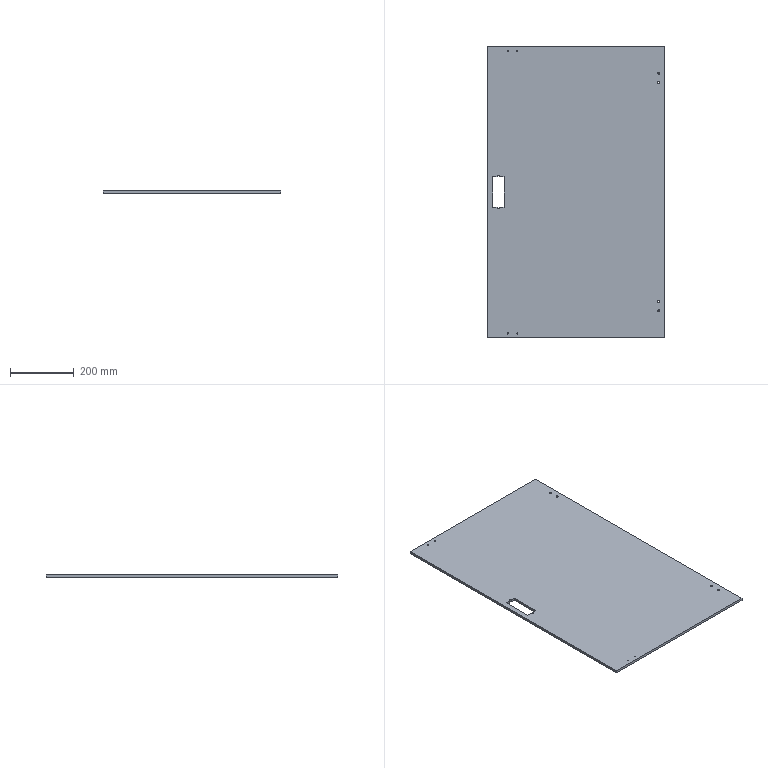Part | STEP file | Right door panel_PN_0006 | 1 solid | 30 faces | box 558 x 917 x 8 mm | volume 4064102 mm3 | cylinder 18 | plane 12 | commonest cylinder face diameters 3.3 x8 6.5 x8 8 x2
STEP:
#1=CARTESIAN_POINT('',(256.75,-373.5,-4.));
#2=VERTEX_POINT('',#1);
#3=CARTESIAN_POINT('',(263.25,-373.5,-4.));
#4=VERTEX_POINT('',#3);
#5=CARTESIAN_POINT('',(260.,-373.5,-4.));
#6=DIRECTION('',(0.,0.,1.));
#7=DIRECTION('',(1.,0.,0.));
#8=AXIS2_PLACEMENT_3D('',#5,#6,#7);
#9=CIRCLE('',#8,3.25);
#10=EDGE_CURVE('',#2,#4,#9,.T.);
#11=ORIENTED_EDGE('',*,*,#10,.F.);
#12=CARTESIAN_POINT('',(256.75,-373.5,4.));
#13=VERTEX_POINT('',#12);
#14=CARTESIAN_POINT('',(256.75,-373.5,-4.));
#15=DIRECTION('',(0.,0.,1.));
#16=VECTOR('',#15,1000.);
#17=LINE('',#14,#16);
#18=EDGE_CURVE('',#2,#13,#17,.T.);
#19=ORIENTED_EDGE('',*,*,#18,.T.);
#20=CARTESIAN_POINT('',(263.25,-373.5,4.));
#21=VERTEX_POINT('',#20);
#22=CARTESIAN_POINT('',(260.,-373.5,4.));
#23=DIRECTION('',(0.,0.,-1.));
#24=DIRECTION('',(1.,0.,0.));
#25=AXIS2_PLACEMENT_3D('',#22,#23,#24);
#26=CIRCLE('',#25,3.25);
#27=EDGE_CURVE('',#21,#13,#26,.T.);
#28=ORIENTED_EDGE('',*,*,#27,.F.);
#29=CARTESIAN_POINT('',(263.25,-373.5,-4.));
#30=DIRECTION('',(0.,0.,1.));
#31=VECTOR('',#30,1000.);
#32=LINE('',#29,#31);
#33=EDGE_CURVE('',#4,#21,#32,.T.);
#34=ORIENTED_EDGE('',*,*,#33,.F.);
#35=EDGE_LOOP('',(#11,#19,#28,#34));
#36=FACE_OUTER_BOUND('',#35,.T.);
#37=CARTESIAN_POINT('',(260.,-373.5,-4.));
#38=DIRECTION('',(0.,0.,1.));
#39=DIRECTION('',(1.,0.,0.));
#40=AXIS2_PLACEMENT_3D('',#37,#38,#39);
#41=CYLINDRICAL_SURFACE('',#40,3.25);
#42=ADVANCED_FACE('',(#36),#41,.F.);
#43=CARTESIAN_POINT('',(256.75,-343.5,-4.));
#44=VERTEX_POINT('',#43);
#45=CARTESIAN_POINT('',(263.25,-343.5,-4.));
#46=VERTEX_POINT('',#45);
#47=CARTESIAN_POINT('',(260.,-343.5,-4.));
#48=DIRECTION('',(0.,0.,1.));
#49=DIRECTION('',(1.,0.,0.));
#50=AXIS2_PLACEMENT_3D('',#47,#48,#49);
#51=CIRCLE('',#50,3.25);
#52=EDGE_CURVE('',#44,#46,#51,.T.);
#53=ORIENTED_EDGE('',*,*,#52,.F.);
#54=CARTESIAN_POINT('',(256.75,-343.5,4.));
#55=VERTEX_POINT('',#54);
#56=CARTESIAN_POINT('',(256.75,-343.5,-4.));
#57=DIRECTION('',(0.,0.,1.));
#58=VECTOR('',#57,1000.);
#59=LINE('',#56,#58);
#60=EDGE_CURVE('',#44,#55,#59,.T.);
#61=ORIENTED_EDGE('',*,*,#60,.T.);
#62=CARTESIAN_POINT('',(263.25,-343.5,4.));
#63=VERTEX_POINT('',#62);
#64=CARTESIAN_POINT('',(260.,-343.5,4.));
#65=DIRECTION('',(0.,0.,-1.));
#66=DIRECTION('',(1.,0.,0.));
#67=AXIS2_PLACEMENT_3D('',#64,#65,#66);
#68=CIRCLE('',#67,3.25);
#69=EDGE_CURVE('',#63,#55,#68,.T.);
#70=ORIENTED_EDGE('',*,*,#69,.F.);
#71=CARTESIAN_POINT('',(263.25,-343.5,-4.));
#72=DIRECTION('',(0.,0.,1.));
#73=VECTOR('',#72,1000.);
#74=LINE('',#71,#73);
#75=EDGE_CURVE('',#46,#63,#74,.T.);
#76=ORIENTED_EDGE('',*,*,#75,.F.);
#77=EDGE_LOOP('',(#53,#61,#70,#76));
#78=FACE_OUTER_BOUND('',#77,.T.);
#79=CARTESIAN_POINT('',(260.,-343.5,-4.));
#80=DIRECTION('',(0.,0.,1.));
#81=DIRECTION('',(1.,0.,0.));
#82=AXIS2_PLACEMENT_3D('',#79,#80,#81);
#83=CYLINDRICAL_SURFACE('',#82,3.25);
#84=ADVANCED_FACE('',(#78),#83,.F.);
#85=CARTESIAN_POINT('',(256.75,343.5,-4.));
#86=VERTEX_POINT('',#85);
#87=CARTESIAN_POINT('',(263.25,343.5,-4.));
#88=VERTEX_POINT('',#87);
#89=CARTESIAN_POINT('',(260.,343.5,-4.));
#90=DIRECTION('',(0.,0.,1.));
#91=DIRECTION('',(1.,0.,0.));
#92=AXIS2_PLACEMENT_3D('',#89,#90,#91);
#93=CIRCLE('',#92,3.25);
#94=EDGE_CURVE('',#86,#88,#93,.T.);
#95=ORIENTED_EDGE('',*,*,#94,.F.);
#96=CARTESIAN_POINT('',(256.75,343.5,4.));
#97=VERTEX_POINT('',#96);
#98=CARTESIAN_POINT('',(256.75,343.5,-4.));
#99=DIRECTION('',(0.,0.,1.));
#100=VECTOR('',#99,1000.);
#101=LINE('',#98,#100);
#102=EDGE_CURVE('',#86,#97,#101,.T.);
#103=ORIENTED_EDGE('',*,*,#102,.T.);
#104=CARTESIAN_POINT('',(263.25,343.5,4.));
#105=VERTEX_POINT('',#104);
#106=CARTESIAN_POINT('',(260.,343.5,4.));
#107=DIRECTION('',(0.,0.,-1.));
#108=DIRECTION('',(1.,0.,0.));
#109=AXIS2_PLACEMENT_3D('',#106,#107,#108);
#110=CIRCLE('',#109,3.25);
#111=EDGE_CURVE('',#105,#97,#110,.T.);
#112=ORIENTED_EDGE('',*,*,#111,.F.);
#113=CARTESIAN_POINT('',(263.25,343.5,-4.));
#114=DIRECTION('',(0.,0.,1.));
#115=VECTOR('',#114,1000.);
#116=LINE('',#113,#115);
#117=EDGE_CURVE('',#88,#105,#116,.T.);
#118=ORIENTED_EDGE('',*,*,#117,.F.);
#119=EDGE_LOOP('',(#95,#103,#112,#118));
#120=FACE_OUTER_BOUND('',#119,.T.);
#121=CARTESIAN_POINT('',(260.,343.5,-4.));
#122=DIRECTION('',(0.,0.,1.));
#123=DIRECTION('',(1.,0.,0.));
#124=AXIS2_PLACEMENT_3D('',#121,#122,#123);
#125=CYLINDRICAL_SURFACE('',#124,3.25);
#126=ADVANCED_FACE('',(#120),#125,.F.);
#127=CARTESIAN_POINT('',(256.75,373.5,-4.));
#128=VERTEX_POINT('',#127);
#129=CARTESIAN_POINT('',(263.25,373.5,-4.));
#130=VERTEX_POINT('',#129);
#131=CARTESIAN_POINT('',(260.,373.5,-4.));
#132=DIRECTION('',(0.,0.,1.));
#133=DIRECTION('',(1.,0.,0.));
#134=AXIS2_PLACEMENT_3D('',#131,#132,#133);
#135=CIRCLE('',#134,3.25);
#136=EDGE_CURVE('',#128,#130,#135,.T.);
#137=ORIENTED_EDGE('',*,*,#136,.F.);
#138=CARTESIAN_POINT('',(256.75,373.5,4.));
#139=VERTEX_POINT('',#138);
#140=CARTESIAN_POINT('',(256.75,373.5,-4.));
#141=DIRECTION('',(0.,0.,1.));
#142=VECTOR('',#141,1000.);
#143=LINE('',#140,#142);
#144=EDGE_CURVE('',#128,#139,#143,.T.);
#145=ORIENTED_EDGE('',*,*,#144,.T.);
#146=CARTESIAN_POINT('',(263.25,373.5,4.));
#147=VERTEX_POINT('',#146);
#148=CARTESIAN_POINT('',(260.,373.5,4.));
#149=DIRECTION('',(0.,0.,-1.));
#150=DIRECTION('',(1.,0.,0.));
#151=AXIS2_PLACEMENT_3D('',#148,#149,#150);
#152=CIRCLE('',#151,3.25);
#153=EDGE_CURVE('',#147,#139,#152,.T.);
#154=ORIENTED_EDGE('',*,*,#153,.F.);
#155=CARTESIAN_POINT('',(263.25,373.5,-4.));
#156=DIRECTION('',(0.,0.,1.));
#157=VECTOR('',#156,1000.);
#158=LINE('',#155,#157);
#159=EDGE_CURVE('',#130,#147,#158,.T.);
#160=ORIENTED_EDGE('',*,*,#159,.F.);
#161=EDGE_LOOP('',(#137,#145,#154,#160));
#162=FACE_OUTER_BOUND('',#161,.T.);
#163=CARTESIAN_POINT('',(260.,373.5,-4.));
#164=DIRECTION('',(0.,0.,1.));
#165=DIRECTION('',(1.,0.,0.));
#166=AXIS2_PLACEMENT_3D('',#163,#164,#165);
#167=CYLINDRICAL_SURFACE('',#166,3.25);
#168=ADVANCED_FACE('',(#162),#167,.F.);
#169=CARTESIAN_POINT('',(-212.35,-444.5,4.));
#170=VERTEX_POINT('',#169);
#171=CARTESIAN_POINT('',(-215.65,-444.5,4.));
#172=VERTEX_POINT('',#171);
#173=CARTESIAN_POINT('',(-214.,-444.5,4.));
#174=DIRECTION('',(0.,0.,-1.));
#175=DIRECTION('',(-1.,0.,0.));
#176=AXIS2_PLACEMENT_3D('',#173,#174,#175);
#177=CIRCLE('',#176,1.65);
#178=EDGE_CURVE('',#170,#172,#177,.T.);
#179=ORIENTED_EDGE('',*,*,#178,.F.);
#180=CARTESIAN_POINT('',(-212.35,-444.5,-4.));
#181=VERTEX_POINT('',#180);
#182=CARTESIAN_POINT('',(-212.35,-444.5,-4.));
#183=DIRECTION('',(0.,0.,-1.));
#184=VECTOR('',#183,1000.);
#185=LINE('',#182,#184);
#186=EDGE_CURVE('',#170,#181,#185,.T.);
#187=ORIENTED_EDGE('',*,*,#186,.T.);
#188=CARTESIAN_POINT('',(-215.65,-444.5,-4.));
#189=VERTEX_POINT('',#188);
#190=CARTESIAN_POINT('',(-214.,-444.5,-4.));
#191=DIRECTION('',(0.,0.,1.));
#192=DIRECTION('',(-1.,0.,0.));
#193=AXIS2_PLACEMENT_3D('',#190,#191,#192);
#194=CIRCLE('',#193,1.65);
#195=EDGE_CURVE('',#189,#181,#194,.T.);
#196=ORIENTED_EDGE('',*,*,#195,.F.);
#197=CARTESIAN_POINT('',(-215.65,-444.5,-4.));
#198=DIRECTION('',(0.,0.,-1.));
#199=VECTOR('',#198,1000.);
#200=LINE('',#197,#199);
#201=EDGE_CURVE('',#172,#189,#200,.T.);
#202=ORIENTED_EDGE('',*,*,#201,.F.);
#203=EDGE_LOOP('',(#179,#187,#196,#202));
#204=FACE_OUTER_BOUND('',#203,.T.);
#205=CARTESIAN_POINT('',(-214.,-444.5,-4.));
#206=DIRECTION('',(0.,0.,-1.));
#207=DIRECTION('',(-1.,0.,0.));
#208=AXIS2_PLACEMENT_3D('',#205,#206,#207);
#209=CYLINDRICAL_SURFACE('',#208,1.65);
#210=ADVANCED_FACE('',(#204),#209,.F.);
#211=CARTESIAN_POINT('',(-182.35,-444.5,4.));
#212=VERTEX_POINT('',#211);
#213=CARTESIAN_POINT('',(-185.65,-444.5,4.));
#214=VERTEX_POINT('',#213);
#215=CARTESIAN_POINT('',(-184.,-444.5,4.));
#216=DIRECTION('',(0.,0.,-1.));
#217=DIRECTION('',(-1.,0.,0.));
#218=AXIS2_PLACEMENT_3D('',#215,#216,#217);
#219=CIRCLE('',#218,1.65);
#220=EDGE_CURVE('',#212,#214,#219,.T.);
#221=ORIENTED_EDGE('',*,*,#220,.F.);
#222=CARTESIAN_POINT('',(-182.35,-444.5,-4.));
#223=VERTEX_POINT('',#222);
#224=CARTESIAN_POINT('',(-182.35,-444.5,-4.));
#225=DIRECTION('',(0.,0.,-1.));
#226=VECTOR('',#225,1000.);
#227=LINE('',#224,#226);
#228=EDGE_CURVE('',#212,#223,#227,.T.);
#229=ORIENTED_EDGE('',*,*,#228,.T.);
#230=CARTESIAN_POINT('',(-185.65,-444.5,-4.));
#231=VERTEX_POINT('',#230);
#232=CARTESIAN_POINT('',(-184.,-444.5,-4.));
#233=DIRECTION('',(0.,0.,1.));
#234=DIRECTION('',(-1.,0.,0.));
#235=AXIS2_PLACEMENT_3D('',#232,#233,#234);
#236=CIRCLE('',#235,1.65);
#237=EDGE_CURVE('',#231,#223,#236,.T.);
#238=ORIENTED_EDGE('',*,*,#237,.F.);
#239=CARTESIAN_POINT('',(-185.65,-444.5,-4.));
#240=DIRECTION('',(0.,0.,-1.));
#241=VECTOR('',#240,1000.);
#242=LINE('',#239,#241);
#243=EDGE_CURVE('',#214,#231,#242,.T.);
#244=ORIENTED_EDGE('',*,*,#243,.F.);
#245=EDGE_LOOP('',(#221,#229,#238,#244));
#246=FACE_OUTER_BOUND('',#245,.T.);
#247=CARTESIAN_POINT('',(-184.,-444.5,-4.));
#248=DIRECTION('',(0.,0.,-1.));
#249=DIRECTION('',(-1.,0.,0.));
#250=AXIS2_PLACEMENT_3D('',#247,#248,#249);
#251=CYLINDRICAL_SURFACE('',#250,1.65);
#252=ADVANCED_FACE('',(#246),#251,.F.);
#253=CARTESIAN_POINT('',(-212.35,443.5,4.));
#254=VERTEX_POINT('',#253);
#255=CARTESIAN_POINT('',(-215.65,443.5,4.));
#256=VERTEX_POINT('',#255);
#257=CARTESIAN_POINT('',(-214.,443.5,4.));
#258=DIRECTION('',(0.,0.,-1.));
#259=DIRECTION('',(-1.,0.,0.));
#260=AXIS2_PLACEMENT_3D('',#257,#258,#259);
#261=CIRCLE('',#260,1.65);
#262=EDGE_CURVE('',#254,#256,#261,.T.);
#263=ORIENTED_EDGE('',*,*,#262,.F.);
#264=CARTESIAN_POINT('',(-212.35,443.5,-4.));
#265=VERTEX_POINT('',#264);
#266=CARTESIAN_POINT('',(-212.35,443.5,-4.));
#267=DIRECTION('',(0.,0.,-1.));
#268=VECTOR('',#267,1000.);
#269=LINE('',#266,#268);
#270=EDGE_CURVE('',#254,#265,#269,.T.);
#271=ORIENTED_EDGE('',*,*,#270,.T.);
#272=CARTESIAN_POINT('',(-215.65,443.5,-4.));
#273=VERTEX_POINT('',#272);
#274=CARTESIAN_POINT('',(-214.,443.5,-4.));
#275=DIRECTION('',(0.,0.,1.));
#276=DIRECTION('',(-1.,0.,0.));
#277=AXIS2_PLACEMENT_3D('',#274,#275,#276);
#278=CIRCLE('',#277,1.65);
#279=EDGE_CURVE('',#273,#265,#278,.T.);
#280=ORIENTED_EDGE('',*,*,#279,.F.);
#281=CARTESIAN_POINT('',(-215.65,443.5,-4.));
#282=DIRECTION('',(0.,0.,-1.));
#283=VECTOR('',#282,1000.);
#284=LINE('',#281,#283);
#285=EDGE_CURVE('',#256,#273,#284,.T.);
#286=ORIENTED_EDGE('',*,*,#285,.F.);
#287=EDGE_LOOP('',(#263,#271,#280,#286));
#288=FACE_OUTER_BOUND('',#287,.T.);
#289=CARTESIAN_POINT('',(-214.,443.5,-4.));
#290=DIRECTION('',(0.,0.,-1.));
#291=DIRECTION('',(-1.,0.,0.));
#292=AXIS2_PLACEMENT_3D('',#289,#290,#291);
#293=CYLINDRICAL_SURFACE('',#292,1.65);
#294=ADVANCED_FACE('',(#288),#293,.F.);
#295=CARTESIAN_POINT('',(-182.35,443.5,4.));
#296=VERTEX_POINT('',#295);
#297=CARTESIAN_POINT('',(-185.65,443.5,4.));
#298=VERTEX_POINT('',#297);
#299=CARTESIAN_POINT('',(-184.,443.5,4.));
#300=DIRECTION('',(0.,0.,-1.));
#301=DIRECTION('',(-1.,0.,0.));
#302=AXIS2_PLACEMENT_3D('',#299,#300,#301);
#303=CIRCLE('',#302,1.65);
#304=EDGE_CURVE('',#296,#298,#303,.T.);
#305=ORIENTED_EDGE('',*,*,#304,.F.);
#306=CARTESIAN_POINT('',(-182.35,443.5,-4.));
#307=VERTEX_POINT('',#306);
#308=CARTESIAN_POINT('',(-182.35,443.5,-4.));
#309=DIRECTION('',(0.,0.,-1.));
#310=VECTOR('',#309,1000.);
#311=LINE('',#308,#310);
#312=EDGE_CURVE('',#296,#307,#311,.T.);
#313=ORIENTED_EDGE('',*,*,#312,.T.);
#314=CARTESIAN_POINT('',(-185.65,443.5,-4.));
#315=VERTEX_POINT('',#314);
#316=CARTESIAN_POINT('',(-184.,443.5,-4.));
#317=DIRECTION('',(0.,0.,1.));
#318=DIRECTION('',(-1.,0.,0.));
#319=AXIS2_PLACEMENT_3D('',#316,#317,#318);
#320=CIRCLE('',#319,1.65);
#321=EDGE_CURVE('',#315,#307,#320,.T.);
#322=ORIENTED_EDGE('',*,*,#321,.F.);
#323=CARTESIAN_POINT('',(-185.65,443.5,-4.));
#324=DIRECTION('',(0.,0.,-1.));
#325=VECTOR('',#324,1000.);
#326=LINE('',#323,#325);
#327=EDGE_CURVE('',#298,#315,#326,.T.);
#328=ORIENTED_EDGE('',*,*,#327,.F.);
#329=EDGE_LOOP('',(#305,#313,#322,#328));
#330=FACE_OUTER_BOUND('',#329,.T.);
#331=CARTESIAN_POINT('',(-184.,443.5,-4.));
#332=DIRECTION('',(0.,0.,-1.));
#333=DIRECTION('',(-1.,0.,0.));
#334=AXIS2_PLACEMENT_3D('',#331,#332,#333);
#335=CYLINDRICAL_SURFACE('',#334,1.65);
#336=ADVANCED_FACE('',(#330),#335,.F.);
#337=CARTESIAN_POINT('',(-262.,-48.,4.));
#338=VERTEX_POINT('',#337);
#339=CARTESIAN_POINT('',(-262.,48.,4.));
#340=VERTEX_POINT('',#339);
#341=CARTESIAN_POINT('',(-262.,0.,4.));
#342=DIRECTION('',(0.,1.,0.));
#343=VECTOR('',#342,1000.);
#344=LINE('',#341,#343);
#345=EDGE_CURVE('',#338,#340,#344,.T.);
#346=ORIENTED_EDGE('',*,*,#345,.T.);
#347=CARTESIAN_POINT('',(-248.,48.,4.));
#348=VERTEX_POINT('',#347);
#349=CARTESIAN_POINT('',(0.,48.,4.));
#350=DIRECTION('',(1.,0.,0.));
#351=VECTOR('',#350,1000.);
#352=LINE('',#349,#351);
#353=EDGE_CURVE('',#340,#348,#352,.T.);
#354=ORIENTED_EDGE('',*,*,#353,.T.);
#355=CARTESIAN_POINT('',(-240.,48.,4.));
#356=VERTEX_POINT('',#355);
#357=CARTESIAN_POINT('',(-244.,48.,4.));
#358=DIRECTION('',(0.,0.,-1.));
#359=DIRECTION('',(1.,0.,0.));
#360=AXIS2_PLACEMENT_3D('',#357,#358,#359);
#361=CIRCLE('',#360,4.);
#362=EDGE_CURVE('',#348,#356,#361,.T.);
#363=ORIENTED_EDGE('',*,*,#362,.T.);
#364=CARTESIAN_POINT('',(-226.,48.,4.));
#365=VERTEX_POINT('',#364);
#366=CARTESIAN_POINT('',(0.,48.,4.));
#367=DIRECTION('',(1.,0.,0.));
#368=VECTOR('',#367,1000.);
#369=LINE('',#366,#368);
#370=EDGE_CURVE('',#356,#365,#369,.T.);
#371=ORIENTED_EDGE('',*,*,#370,.T.);
#372=CARTESIAN_POINT('',(-226.,-48.,4.));
#373=VERTEX_POINT('',#372);
#374=CARTESIAN_POINT('',(-226.,0.,4.));
#375=DIRECTION('',(0.,-1.,0.));
#376=VECTOR('',#375,1000.);
#377=LINE('',#374,#376);
#378=EDGE_CURVE('',#365,#373,#377,.T.);
#379=ORIENTED_EDGE('',*,*,#378,.T.);
#380=CARTESIAN_POINT('',(-240.,-48.,4.));
#381=VERTEX_POINT('',#380);
#382=CARTESIAN_POINT('',(0.,-48.,4.));
#383=DIRECTION('',(-1.,0.,0.));
#384=VECTOR('',#383,1000.);
#385=LINE('',#382,#384);
#386=EDGE_CURVE('',#373,#381,#385,.T.);
#387=ORIENTED_EDGE('',*,*,#386,.T.);
#388=CARTESIAN_POINT('',(-248.,-48.,4.));
#389=VERTEX_POINT('',#388);
#390=CARTESIAN_POINT('',(-244.,-48.,4.));
#391=DIRECTION('',(0.,0.,-1.));
#392=DIRECTION('',(1.,0.,0.));
#393=AXIS2_PLACEMENT_3D('',#390,#391,#392);
#394=CIRCLE('',#393,4.);
#395=EDGE_CURVE('',#381,#389,#394,.T.);
#396=ORIENTED_EDGE('',*,*,#395,.T.);
#397=CARTESIAN_POINT('',(0.,-48.,4.));
#398=DIRECTION('',(-1.,0.,0.));
#399=VECTOR('',#398,1000.);
#400=LINE('',#397,#399);
#401=EDGE_CURVE('',#389,#338,#400,.T.);
#402=ORIENTED_EDGE('',*,*,#401,.T.);
#403=EDGE_LOOP('',(#346,#354,#363,#371,#379,#387,#396,#402));
#404=FACE_BOUND('',#403,.T.);
#405=CARTESIAN_POINT('',(-279.,458.5,4.));
#406=VERTEX_POINT('',#405);
#407=CARTESIAN_POINT('',(-279.,-458.5,4.));
#408=VERTEX_POINT('',#407);
#409=CARTESIAN_POINT('',(-279.,0.,4.));
#410=DIRECTION('',(0.,-1.,0.));
#411=VECTOR('',#410,1000.);
#412=LINE('',#409,#411);
#413=EDGE_CURVE('',#406,#408,#412,.T.);
#414=ORIENTED_EDGE('',*,*,#413,.T.);
#415=CARTESIAN_POINT('',(279.,-458.5,4.));
#416=VERTEX_POINT('',#415);
#417=CARTESIAN_POINT('',(0.,-458.5,4.));
#418=DIRECTION('',(1.,0.,0.));
#419=VECTOR('',#418,1000.);
#420=LINE('',#417,#419);
#421=EDGE_CURVE('',#408,#416,#420,.T.);
#422=ORIENTED_EDGE('',*,*,#421,.T.);
#423=CARTESIAN_POINT('',(279.,458.5,4.));
#424=VERTEX_POINT('',#423);
#425=CARTESIAN_POINT('',(279.,0.,4.));
#426=DIRECTION('',(0.,1.,0.));
#427=VECTOR('',#426,1000.);
#428=LINE('',#425,#427);
#429=EDGE_CURVE('',#416,#424,#428,.T.);
#430=ORIENTED_EDGE('',*,*,#429,.T.);
#431=CARTESIAN_POINT('',(0.,458.5,4.));
#432=DIRECTION('',(-1.,0.,0.));
#433=VECTOR('',#432,1000.);
#434=LINE('',#431,#433);
#435=EDGE_CURVE('',#424,#406,#434,.T.);
#436=ORIENTED_EDGE('',*,*,#435,.T.);
#437=EDGE_LOOP('',(#414,#422,#430,#436));
#438=FACE_OUTER_BOUND('',#437,.T.);
#439=ORIENTED_EDGE('',*,*,#27,.T.);
#440=CARTESIAN_POINT('',(260.,-373.5,4.));
#441=DIRECTION('',(0.,0.,-1.));
#442=DIRECTION('',(1.,0.,0.));
#443=AXIS2_PLACEMENT_3D('',#440,#441,#442);
#444=CIRCLE('',#443,3.25);
#445=EDGE_CURVE('',#13,#21,#444,.T.);
#446=ORIENTED_EDGE('',*,*,#445,.T.);
#447=EDGE_LOOP('',(#439,#446));
#448=FACE_BOUND('',#447,.T.);
#449=ORIENTED_EDGE('',*,*,#69,.T.);
#450=CARTESIAN_POINT('',(260.,-343.5,4.));
#451=DIRECTION('',(0.,0.,-1.));
#452=DIRECTION('',(1.,0.,0.));
#453=AXIS2_PLACEMENT_3D('',#450,#451,#452);
#454=CIRCLE('',#453,3.25);
#455=EDGE_CURVE('',#55,#63,#454,.T.);
#456=ORIENTED_EDGE('',*,*,#455,.T.);
#457=EDGE_LOOP('',(#449,#456));
#458=FACE_BOUND('',#457,.T.);
#459=ORIENTED_EDGE('',*,*,#111,.T.);
#460=CARTESIAN_POINT('',(260.,343.5,4.));
#461=DIRECTION('',(0.,0.,-1.));
#462=DIRECTION('',(1.,0.,0.));
#463=AXIS2_PLACEMENT_3D('',#460,#461,#462);
#464=CIRCLE('',#463,3.25);
#465=EDGE_CURVE('',#97,#105,#464,.T.);
#466=ORIENTED_EDGE('',*,*,#465,.T.);
#467=EDGE_LOOP('',(#459,#466));
#468=FACE_BOUND('',#467,.T.);
#469=ORIENTED_EDGE('',*,*,#153,.T.);
#470=CARTESIAN_POINT('',(260.,373.5,4.));
#471=DIRECTION('',(0.,0.,-1.));
#472=DIRECTION('',(1.,0.,0.));
#473=AXIS2_PLACEMENT_3D('',#470,#471,#472);
#474=CIRCLE('',#473,3.25);
#475=EDGE_CURVE('',#139,#147,#474,.T.);
#476=ORIENTED_EDGE('',*,*,#475,.T.);
#477=EDGE_LOOP('',(#469,#476));
#478=FACE_BOUND('',#477,.T.);
#479=CARTESIAN_POINT('',(-214.,-444.5,4.));
#480=DIRECTION('',(0.,0.,-1.));
#481=DIRECTION('',(-1.,0.,0.));
#482=AXIS2_PLACEMENT_3D('',#479,#480,#481);
#483=CIRCLE('',#482,1.65);
#484=EDGE_CURVE('',#172,#170,#483,.T.);
#485=ORIENTED_EDGE('',*,*,#484,.T.);
#486=ORIENTED_EDGE('',*,*,#178,.T.);
#487=EDGE_LOOP('',(#485,#486));
#488=FACE_BOUND('',#487,.T.);
#489=CARTESIAN_POINT('',(-184.,-444.5,4.));
#490=DIRECTION('',(0.,0.,-1.));
#491=DIRECTION('',(-1.,0.,0.));
#492=AXIS2_PLACEMENT_3D('',#489,#490,#491);
#493=CIRCLE('',#492,1.65);
#494=EDGE_CURVE('',#214,#212,#493,.T.);
#495=ORIENTED_EDGE('',*,*,#494,.T.);
#496=ORIENTED_EDGE('',*,*,#220,.T.);
#497=EDGE_LOOP('',(#495,#496));
#498=FACE_BOUND('',#497,.T.);
#499=CARTESIAN_POINT('',(-214.,443.5,4.));
#500=DIRECTION('',(0.,0.,-1.));
#501=DIRECTION('',(-1.,0.,0.));
#502=AXIS2_PLACEMENT_3D('',#499,#500,#501);
#503=CIRCLE('',#502,1.65);
#504=EDGE_CURVE('',#256,#254,#503,.T.);
#505=ORIENTED_EDGE('',*,*,#504,.T.);
#506=ORIENTED_EDGE('',*,*,#262,.T.);
#507=EDGE_LOOP('',(#505,#506));
#508=FACE_BOUND('',#507,.T.);
#509=CARTESIAN_POINT('',(-184.,443.5,4.));
#510=DIRECTION('',(0.,0.,-1.));
#511=DIRECTION('',(-1.,0.,0.));
#512=AXIS2_PLACEMENT_3D('',#509,#510,#511);
#513=CIRCLE('',#512,1.65);
#514=EDGE_CURVE('',#298,#296,#513,.T.);
#515=ORIENTED_EDGE('',*,*,#514,.T.);
#516=ORIENTED_EDGE('',*,*,#304,.T.);
#517=EDGE_LOOP('',(#515,#516));
#518=FACE_BOUND('',#517,.T.);
#519=CARTESIAN_POINT('',(0.,0.,4.));
#520=DIRECTION('',(0.,0.,1.));
#521=DIRECTION('',(1.,0.,0.));
#522=AXIS2_PLACEMENT_3D('',#519,#520,#521);
#523=PLANE('',#522);
#524=ADVANCED_FACE('',(#404,#438,#448,#458,#468,#478,#488,#498,#508,#518),#523,.T.);
#525=CARTESIAN_POINT('',(-262.,48.,-4.));
#526=VERTEX_POINT('',#525);
#527=CARTESIAN_POINT('',(-248.,48.,-4.));
#528=VERTEX_POINT('',#527);
#529=CARTESIAN_POINT('',(0.,48.,-4.));
#530=DIRECTION('',(1.,0.,0.));
#531=VECTOR('',#530,1000.);
#532=LINE('',#529,#531);
#533=EDGE_CURVE('',#526,#528,#532,.T.);
#534=ORIENTED_EDGE('',*,*,#533,.T.);
#535=CARTESIAN_POINT('',(-248.,48.,-4.));
#536=DIRECTION('',(0.,0.,1.));
#537=VECTOR('',#536,1000.);
#538=LINE('',#535,#537);
#539=EDGE_CURVE('',#528,#348,#538,.T.);
#540=ORIENTED_EDGE('',*,*,#539,.T.);
#541=ORIENTED_EDGE('',*,*,#353,.F.);
#542=CARTESIAN_POINT('',(-262.,48.,-4.));
#543=DIRECTION('',(0.,0.,-1.));
#544=VECTOR('',#543,1000.);
#545=LINE('',#542,#544);
#546=EDGE_CURVE('',#340,#526,#545,.T.);
#547=ORIENTED_EDGE('',*,*,#546,.T.);
#548=EDGE_LOOP('',(#534,#540,#541,#547));
#549=FACE_OUTER_BOUND('',#548,.T.);
#550=CARTESIAN_POINT('',(0.,48.,-4.));
#551=DIRECTION('',(0.,-1.,0.));
#552=DIRECTION('',(0.,0.,-1.));
#553=AXIS2_PLACEMENT_3D('',#550,#551,#552);
#554=PLANE('',#553);
#555=ADVANCED_FACE('',(#549),#554,.T.);
#556=CARTESIAN_POINT('',(-262.,-48.,-4.));
#557=VERTEX_POINT('',#556);
#558=CARTESIAN_POINT('',(-262.,-48.,-4.));
#559=DIRECTION('',(0.,0.,1.));
#560=VECTOR('',#559,1000.);
#561=LINE('',#558,#560);
#562=EDGE_CURVE('',#557,#338,#561,.T.);
#563=ORIENTED_EDGE('',*,*,#562,.F.);
#564=CARTESIAN_POINT('',(-262.,0.,-4.));
#565=DIRECTION('',(0.,-1.,0.));
#566=VECTOR('',#565,1000.);
#567=LINE('',#564,#566);
#568=EDGE_CURVE('',#526,#557,#567,.T.);
#569=ORIENTED_EDGE('',*,*,#568,.F.);
#570=ORIENTED_EDGE('',*,*,#546,.F.);
#571=ORIENTED_EDGE('',*,*,#345,.F.);
#572=EDGE_LOOP('',(#563,#569,#570,#571));
#573=FACE_OUTER_BOUND('',#572,.T.);
#574=CARTESIAN_POINT('',(-262.,0.,-4.));
#575=DIRECTION('',(-1.,0.,0.));
#576=DIRECTION('',(0.,0.,1.));
#577=AXIS2_PLACEMENT_3D('',#574,#575,#576);
#578=PLANE('',#577);
#579=ADVANCED_FACE('',(#573),#578,.F.);
#580=CARTESIAN_POINT('',(-248.,-48.,-4.));
#581=VERTEX_POINT('',#580);
#582=CARTESIAN_POINT('',(-248.,-48.,-4.));
#583=DIRECTION('',(0.,0.,1.));
#584=VECTOR('',#583,1000.);
#585=LINE('',#582,#584);
#586=EDGE_CURVE('',#581,#389,#585,.T.);
#587=ORIENTED_EDGE('',*,*,#586,.F.);
#588=CARTESIAN_POINT('',(0.,-48.,-4.));
#589=DIRECTION('',(1.,0.,0.));
#590=VECTOR('',#589,1000.);
#591=LINE('',#588,#590);
#592=EDGE_CURVE('',#557,#581,#591,.T.);
#593=ORIENTED_EDGE('',*,*,#592,.F.);
#594=ORIENTED_EDGE('',*,*,#562,.T.);
#595=ORIENTED_EDGE('',*,*,#401,.F.);
#596=EDGE_LOOP('',(#587,#593,#594,#595));
#597=FACE_OUTER_BOUND('',#596,.T.);
#598=CARTESIAN_POINT('',(0.,-48.,-4.));
#599=DIRECTION('',(0.,-1.,0.));
#600=DIRECTION('',(0.,0.,-1.));
#601=AXIS2_PLACEMENT_3D('',#598,#599,#600);
#602=PLANE('',#601);
#603=ADVANCED_FACE('',(#597),#602,.F.);
#604=CARTESIAN_POINT('',(-240.,-48.,-4.));
#605=VERTEX_POINT('',#604);
#606=CARTESIAN_POINT('',(-240.,-48.,-4.));
#607=DIRECTION('',(0.,0.,1.));
#608=VECTOR('',#607,1000.);
#609=LINE('',#606,#608);
#610=EDGE_CURVE('',#605,#381,#609,.T.);
#611=ORIENTED_EDGE('',*,*,#610,.F.);
#612=CARTESIAN_POINT('',(-244.,-48.,-4.));
#613=DIRECTION('',(0.,0.,1.));
#614=DIRECTION('',(1.,0.,0.));
#615=AXIS2_PLACEMENT_3D('',#612,#613,#614);
#616=CIRCLE('',#615,4.);
#617=EDGE_CURVE('',#581,#605,#616,.T.);
#618=ORIENTED_EDGE('',*,*,#617,.F.);
#619=ORIENTED_EDGE('',*,*,#586,.T.);
#620=ORIENTED_EDGE('',*,*,#395,.F.);
#621=EDGE_LOOP('',(#611,#618,#619,#620));
#622=FACE_OUTER_BOUND('',#621,.T.);
#623=CARTESIAN_POINT('',(-244.,-48.,-4.));
#624=DIRECTION('',(0.,0.,1.));
#625=DIRECTION('',(1.,0.,0.));
#626=AXIS2_PLACEMENT_3D('',#623,#624,#625);
#627=CYLINDRICAL_SURFACE('',#626,4.);
#628=ADVANCED_FACE('',(#622),#627,.F.);
#629=CARTESIAN_POINT('',(-226.,-48.,-4.));
#630=VERTEX_POINT('',#629);
#631=CARTESIAN_POINT('',(-226.,-48.,-4.));
#632=DIRECTION('',(0.,0.,1.));
#633=VECTOR('',#632,1000.);
#634=LINE('',#631,#633);
#635=EDGE_CURVE('',#630,#373,#634,.T.);
#636=ORIENTED_EDGE('',*,*,#635,.F.);
#637=CARTESIAN_POINT('',(0.,-48.,-4.));
#638=DIRECTION('',(1.,0.,0.));
#639=VECTOR('',#638,1000.);
#640=LINE('',#637,#639);
#641=EDGE_CURVE('',#605,#630,#640,.T.);
#642=ORIENTED_EDGE('',*,*,#641,.F.);
#643=ORIENTED_EDGE('',*,*,#610,.T.);
#644=ORIENTED_EDGE('',*,*,#386,.F.);
#645=EDGE_LOOP('',(#636,#642,#643,#644));
#646=FACE_OUTER_BOUND('',#645,.T.);
#647=CARTESIAN_POINT('',(0.,-48.,-4.));
#648=DIRECTION('',(0.,-1.,0.));
#649=DIRECTION('',(0.,0.,-1.));
#650=AXIS2_PLACEMENT_3D('',#647,#648,#649);
#651=PLANE('',#650);
#652=ADVANCED_FACE('',(#646),#651,.F.);
#653=CARTESIAN_POINT('',(-226.,48.,-4.));
#654=VERTEX_POINT('',#653);
#655=CARTESIAN_POINT('',(-226.,0.,-4.));
#656=DIRECTION('',(0.,-1.,0.));
#657=VECTOR('',#656,1000.);
#658=LINE('',#655,#657);
#659=EDGE_CURVE('',#654,#630,#658,.T.);
#660=ORIENTED_EDGE('',*,*,#659,.T.);
#661=ORIENTED_EDGE('',*,*,#635,.T.);
#662=ORIENTED_EDGE('',*,*,#378,.F.);
#663=CARTESIAN_POINT('',(-226.,48.,-4.));
#664=DIRECTION('',(0.,0.,-1.));
#665=VECTOR('',#664,1000.);
#666=LINE('',#663,#665);
#667=EDGE_CURVE('',#365,#654,#666,.T.);
#668=ORIENTED_EDGE('',*,*,#667,.T.);
#669=EDGE_LOOP('',(#660,#661,#662,#668));
#670=FACE_OUTER_BOUND('',#669,.T.);
#671=CARTESIAN_POINT('',(-226.,0.,-4.));
#672=DIRECTION('',(-1.,0.,0.));
#673=DIRECTION('',(0.,0.,1.));
#674=AXIS2_PLACEMENT_3D('',#671,#672,#673);
#675=PLANE('',#674);
#676=ADVANCED_FACE('',(#670),#675,.T.);
#677=CARTESIAN_POINT('',(-240.,48.,-4.));
#678=VERTEX_POINT('',#677);
#679=CARTESIAN_POINT('',(0.,48.,-4.));
#680=DIRECTION('',(1.,0.,0.));
#681=VECTOR('',#680,1000.);
#682=LINE('',#679,#681);
#683=EDGE_CURVE('',#678,#654,#682,.T.);
#684=ORIENTED_EDGE('',*,*,#683,.T.);
#685=ORIENTED_EDGE('',*,*,#667,.F.);
#686=ORIENTED_EDGE('',*,*,#370,.F.);
#687=CARTESIAN_POINT('',(-240.,48.,-4.));
#688=DIRECTION('',(0.,0.,-1.));
#689=VECTOR('',#688,1000.);
#690=LINE('',#687,#689);
#691=EDGE_CURVE('',#356,#678,#690,.T.);
#692=ORIENTED_EDGE('',*,*,#691,.T.);
#693=EDGE_LOOP('',(#684,#685,#686,#692));
#694=FACE_OUTER_BOUND('',#693,.T.);
#695=CARTESIAN_POINT('',(0.,48.,-4.));
#696=DIRECTION('',(0.,-1.,0.));
#697=DIRECTION('',(0.,0.,-1.));
#698=AXIS2_PLACEMENT_3D('',#695,#696,#697);
#699=PLANE('',#698);
#700=ADVANCED_FACE('',(#694),#699,.T.);
#701=ORIENTED_EDGE('',*,*,#539,.F.);
#702=CARTESIAN_POINT('',(-244.,48.,-4.));
#703=DIRECTION('',(0.,0.,1.));
#704=DIRECTION('',(1.,0.,0.));
#705=AXIS2_PLACEMENT_3D('',#702,#703,#704);
#706=CIRCLE('',#705,4.);
#707=EDGE_CURVE('',#678,#528,#706,.T.);
#708=ORIENTED_EDGE('',*,*,#707,.F.);
#709=ORIENTED_EDGE('',*,*,#691,.F.);
#710=ORIENTED_EDGE('',*,*,#362,.F.);
#711=EDGE_LOOP('',(#701,#708,#709,#710));
#712=FACE_OUTER_BOUND('',#711,.T.);
#713=CARTESIAN_POINT('',(-244.,48.,-4.));
#714=DIRECTION('',(0.,0.,1.));
#715=DIRECTION('',(1.,0.,0.));
#716=AXIS2_PLACEMENT_3D('',#713,#714,#715);
#717=CYLINDRICAL_SURFACE('',#716,4.);
#718=ADVANCED_FACE('',(#712),#717,.F.);
#719=CARTESIAN_POINT('',(279.,-458.5,-4.));
#720=VERTEX_POINT('',#719);
#721=CARTESIAN_POINT('',(279.,-458.5,4.));
#722=DIRECTION('',(0.,0.,-1.));
#723=VECTOR('',#722,1000.);
#724=LINE('',#721,#723);
#725=EDGE_CURVE('',#416,#720,#724,.T.);
#726=ORIENTED_EDGE('',*,*,#725,.F.);
#727=ORIENTED_EDGE('',*,*,#421,.F.);
#728=CARTESIAN_POINT('',(-279.,-458.5,-4.));
#729=VERTEX_POINT('',#728);
#730=CARTESIAN_POINT('',(-279.,-458.5,4.));
#731=DIRECTION('',(0.,0.,1.));
#732=VECTOR('',#731,1000.);
#733=LINE('',#730,#732);
#734=EDGE_CURVE('',#729,#408,#733,.T.);
#735=ORIENTED_EDGE('',*,*,#734,.F.);
#736=CARTESIAN_POINT('',(-279.,-458.5,-4.));
#737=DIRECTION('',(-1.,0.,0.));
#738=VECTOR('',#737,1000.);
#739=LINE('',#736,#738);
#740=EDGE_CURVE('',#720,#729,#739,.T.);
#741=ORIENTED_EDGE('',*,*,#740,.F.);
#742=EDGE_LOOP('',(#726,#727,#735,#741));
#743=FACE_OUTER_BOUND('',#742,.T.);
#744=CARTESIAN_POINT('',(-279.,-458.5,4.));
#745=DIRECTION('',(0.,1.,0.));
#746=DIRECTION('',(0.,0.,1.));
#747=AXIS2_PLACEMENT_3D('',#744,#745,#746);
#748=PLANE('',#747);
#749=ADVANCED_FACE('',(#743),#748,.F.);
#750=ORIENTED_EDGE('',*,*,#734,.T.);
#751=ORIENTED_EDGE('',*,*,#413,.F.);
#752=CARTESIAN_POINT('',(-279.,458.5,-4.));
#753=VERTEX_POINT('',#752);
#754=CARTESIAN_POINT('',(-279.,458.5,4.));
#755=DIRECTION('',(0.,0.,1.));
#756=VECTOR('',#755,1000.);
#757=LINE('',#754,#756);
#758=EDGE_CURVE('',#753,#406,#757,.T.);
#759=ORIENTED_EDGE('',*,*,#758,.F.);
#760=CARTESIAN_POINT('',(-279.,458.5,-4.));
#761=DIRECTION('',(0.,1.,0.));
#762=VECTOR('',#761,1000.);
#763=LINE('',#760,#762);
#764=EDGE_CURVE('',#729,#753,#763,.T.);
#765=ORIENTED_EDGE('',*,*,#764,.F.);
#766=EDGE_LOOP('',(#750,#751,#759,#765));
#767=FACE_OUTER_BOUND('',#766,.T.);
#768=CARTESIAN_POINT('',(-279.,458.5,4.));
#769=DIRECTION('',(1.,0.,0.));
#770=DIRECTION('',(0.,1.,0.));
#771=AXIS2_PLACEMENT_3D('',#768,#769,#770);
#772=PLANE('',#771);
#773=ADVANCED_FACE('',(#767),#772,.F.);
#774=ORIENTED_EDGE('',*,*,#758,.T.);
#775=ORIENTED_EDGE('',*,*,#435,.F.);
#776=CARTESIAN_POINT('',(279.,458.5,-4.));
#777=VERTEX_POINT('',#776);
#778=CARTESIAN_POINT('',(279.,458.5,4.));
#779=DIRECTION('',(0.,0.,1.));
#780=VECTOR('',#779,1000.);
#781=LINE('',#778,#780);
#782=EDGE_CURVE('',#777,#424,#781,.T.);
#783=ORIENTED_EDGE('',*,*,#782,.F.);
#784=CARTESIAN_POINT('',(-279.,458.5,-4.));
#785=DIRECTION('',(1.,0.,0.));
#786=VECTOR('',#785,1000.);
#787=LINE('',#784,#786);
#788=EDGE_CURVE('',#753,#777,#787,.T.);
#789=ORIENTED_EDGE('',*,*,#788,.F.);
#790=EDGE_LOOP('',(#774,#775,#783,#789));
#791=FACE_OUTER_BOUND('',#790,.T.);
#792=CARTESIAN_POINT('',(-279.,458.5,4.));
#793=DIRECTION('',(0.,-1.,0.));
#794=DIRECTION('',(0.,0.,-1.));
#795=AXIS2_PLACEMENT_3D('',#792,#793,#794);
#796=PLANE('',#795);
#797=ADVANCED_FACE('',(#791),#796,.F.);
#798=ORIENTED_EDGE('',*,*,#782,.T.);
#799=ORIENTED_EDGE('',*,*,#429,.F.);
#800=ORIENTED_EDGE('',*,*,#725,.T.);
#801=CARTESIAN_POINT('',(279.,458.5,-4.));
#802=DIRECTION('',(0.,-1.,0.));
#803=VECTOR('',#802,1000.);
#804=LINE('',#801,#803);
#805=EDGE_CURVE('',#777,#720,#804,.T.);
#806=ORIENTED_EDGE('',*,*,#805,.F.);
#807=EDGE_LOOP('',(#798,#799,#800,#806));
#808=FACE_OUTER_BOUND('',#807,.T.);
#809=CARTESIAN_POINT('',(279.,458.5,4.));
#810=DIRECTION('',(-1.,0.,0.));
#811=DIRECTION('',(0.,-1.,0.));
#812=AXIS2_PLACEMENT_3D('',#809,#810,#811);
#813=PLANE('',#812);
#814=ADVANCED_FACE('',(#808),#813,.F.);
#815=ORIENTED_EDGE('',*,*,#18,.F.);
#816=CARTESIAN_POINT('',(260.,-373.5,-4.));
#817=DIRECTION('',(0.,0.,1.));
#818=DIRECTION('',(1.,0.,0.));
#819=AXIS2_PLACEMENT_3D('',#816,#817,#818);
#820=CIRCLE('',#819,3.25);
#821=EDGE_CURVE('',#4,#2,#820,.T.);
#822=ORIENTED_EDGE('',*,*,#821,.F.);
#823=ORIENTED_EDGE('',*,*,#33,.T.);
#824=ORIENTED_EDGE('',*,*,#445,.F.);
#825=EDGE_LOOP('',(#815,#822,#823,#824));
#826=FACE_OUTER_BOUND('',#825,.T.);
#827=CARTESIAN_POINT('',(260.,-373.5,-4.));
#828=DIRECTION('',(0.,0.,1.));
#829=DIRECTION('',(1.,0.,0.));
#830=AXIS2_PLACEMENT_3D('',#827,#828,#829);
#831=CYLINDRICAL_SURFACE('',#830,3.25);
#832=ADVANCED_FACE('',(#826),#831,.F.);
#833=ORIENTED_EDGE('',*,*,#60,.F.);
#834=CARTESIAN_POINT('',(260.,-343.5,-4.));
#835=DIRECTION('',(0.,0.,1.));
#836=DIRECTION('',(1.,0.,0.));
#837=AXIS2_PLACEMENT_3D('',#834,#835,#836);
#838=CIRCLE('',#837,3.25);
#839=EDGE_CURVE('',#46,#44,#838,.T.);
#840=ORIENTED_EDGE('',*,*,#839,.F.);
#841=ORIENTED_EDGE('',*,*,#75,.T.);
#842=ORIENTED_EDGE('',*,*,#455,.F.);
#843=EDGE_LOOP('',(#833,#840,#841,#842));
#844=FACE_OUTER_BOUND('',#843,.T.);
#845=CARTESIAN_POINT('',(260.,-343.5,-4.));
#846=DIRECTION('',(0.,0.,1.));
#847=DIRECTION('',(1.,0.,0.));
#848=AXIS2_PLACEMENT_3D('',#845,#846,#847);
#849=CYLINDRICAL_SURFACE('',#848,3.25);
#850=ADVANCED_FACE('',(#844),#849,.F.);
#851=ORIENTED_EDGE('',*,*,#102,.F.);
#852=CARTESIAN_POINT('',(260.,343.5,-4.));
#853=DIRECTION('',(0.,0.,1.));
#854=DIRECTION('',(1.,0.,0.));
#855=AXIS2_PLACEMENT_3D('',#852,#853,#854);
#856=CIRCLE('',#855,3.25);
#857=EDGE_CURVE('',#88,#86,#856,.T.);
#858=ORIENTED_EDGE('',*,*,#857,.F.);
#859=ORIENTED_EDGE('',*,*,#117,.T.);
#860=ORIENTED_EDGE('',*,*,#465,.F.);
#861=EDGE_LOOP('',(#851,#858,#859,#860));
#862=FACE_OUTER_BOUND('',#861,.T.);
#863=CARTESIAN_POINT('',(260.,343.5,-4.));
#864=DIRECTION('',(0.,0.,1.));
#865=DIRECTION('',(1.,0.,0.));
#866=AXIS2_PLACEMENT_3D('',#863,#864,#865);
#867=CYLINDRICAL_SURFACE('',#866,3.25);
#868=ADVANCED_FACE('',(#862),#867,.F.);
#869=ORIENTED_EDGE('',*,*,#144,.F.);
#870=CARTESIAN_POINT('',(260.,373.5,-4.));
#871=DIRECTION('',(0.,0.,1.));
#872=DIRECTION('',(1.,0.,0.));
#873=AXIS2_PLACEMENT_3D('',#870,#871,#872);
#874=CIRCLE('',#873,3.25);
#875=EDGE_CURVE('',#130,#128,#874,.T.);
#876=ORIENTED_EDGE('',*,*,#875,.F.);
#877=ORIENTED_EDGE('',*,*,#159,.T.);
#878=ORIENTED_EDGE('',*,*,#475,.F.);
#879=EDGE_LOOP('',(#869,#876,#877,#878));
#880=FACE_OUTER_BOUND('',#879,.T.);
#881=CARTESIAN_POINT('',(260.,373.5,-4.));
#882=DIRECTION('',(0.,0.,1.));
#883=DIRECTION('',(1.,0.,0.));
#884=AXIS2_PLACEMENT_3D('',#881,#882,#883);
#885=CYLINDRICAL_SURFACE('',#884,3.25);
#886=ADVANCED_FACE('',(#880),#885,.F.);
#887=ORIENTED_EDGE('',*,*,#186,.F.);
#888=ORIENTED_EDGE('',*,*,#484,.F.);
#889=ORIENTED_EDGE('',*,*,#201,.T.);
#890=CARTESIAN_POINT('',(-214.,-444.5,-4.));
#891=DIRECTION('',(0.,0.,1.));
#892=DIRECTION('',(-1.,0.,0.));
#893=AXIS2_PLACEMENT_3D('',#890,#891,#892);
#894=CIRCLE('',#893,1.65);
#895=EDGE_CURVE('',#181,#189,#894,.T.);
#896=ORIENTED_EDGE('',*,*,#895,.F.);
#897=EDGE_LOOP('',(#887,#888,#889,#896));
#898=FACE_OUTER_BOUND('',#897,.T.);
#899=CARTESIAN_POINT('',(-214.,-444.5,-4.));
#900=DIRECTION('',(0.,0.,-1.));
#901=DIRECTION('',(-1.,0.,0.));
#902=AXIS2_PLACEMENT_3D('',#899,#900,#901);
#903=CYLINDRICAL_SURFACE('',#902,1.65);
#904=ADVANCED_FACE('',(#898),#903,.F.);
#905=ORIENTED_EDGE('',*,*,#228,.F.);
#906=ORIENTED_EDGE('',*,*,#494,.F.);
#907=ORIENTED_EDGE('',*,*,#243,.T.);
#908=CARTESIAN_POINT('',(-184.,-444.5,-4.));
#909=DIRECTION('',(0.,0.,1.));
#910=DIRECTION('',(-1.,0.,0.));
#911=AXIS2_PLACEMENT_3D('',#908,#909,#910);
#912=CIRCLE('',#911,1.65);
#913=EDGE_CURVE('',#223,#231,#912,.T.);
#914=ORIENTED_EDGE('',*,*,#913,.F.);
#915=EDGE_LOOP('',(#905,#906,#907,#914));
#916=FACE_OUTER_BOUND('',#915,.T.);
#917=CARTESIAN_POINT('',(-184.,-444.5,-4.));
#918=DIRECTION('',(0.,0.,-1.));
#919=DIRECTION('',(-1.,0.,0.));
#920=AXIS2_PLACEMENT_3D('',#917,#918,#919);
#921=CYLINDRICAL_SURFACE('',#920,1.65);
#922=ADVANCED_FACE('',(#916),#921,.F.);
#923=ORIENTED_EDGE('',*,*,#270,.F.);
#924=ORIENTED_EDGE('',*,*,#504,.F.);
#925=ORIENTED_EDGE('',*,*,#285,.T.);
#926=CARTESIAN_POINT('',(-214.,443.5,-4.));
#927=DIRECTION('',(0.,0.,1.));
#928=DIRECTION('',(-1.,0.,0.));
#929=AXIS2_PLACEMENT_3D('',#926,#927,#928);
#930=CIRCLE('',#929,1.65);
#931=EDGE_CURVE('',#265,#273,#930,.T.);
#932=ORIENTED_EDGE('',*,*,#931,.F.);
#933=EDGE_LOOP('',(#923,#924,#925,#932));
#934=FACE_OUTER_BOUND('',#933,.T.);
#935=CARTESIAN_POINT('',(-214.,443.5,-4.));
#936=DIRECTION('',(0.,0.,-1.));
#937=DIRECTION('',(-1.,0.,0.));
#938=AXIS2_PLACEMENT_3D('',#935,#936,#937);
#939=CYLINDRICAL_SURFACE('',#938,1.65);
#940=ADVANCED_FACE('',(#934),#939,.F.);
#941=ORIENTED_EDGE('',*,*,#312,.F.);
#942=ORIENTED_EDGE('',*,*,#514,.F.);
#943=ORIENTED_EDGE('',*,*,#327,.T.);
#944=CARTESIAN_POINT('',(-184.,443.5,-4.));
#945=DIRECTION('',(0.,0.,1.));
#946=DIRECTION('',(-1.,0.,0.));
#947=AXIS2_PLACEMENT_3D('',#944,#945,#946);
#948=CIRCLE('',#947,1.65);
#949=EDGE_CURVE('',#307,#315,#948,.T.);
#950=ORIENTED_EDGE('',*,*,#949,.F.);
#951=EDGE_LOOP('',(#941,#942,#943,#950));
#952=FACE_OUTER_BOUND('',#951,.T.);
#953=CARTESIAN_POINT('',(-184.,443.5,-4.));
#954=DIRECTION('',(0.,0.,-1.));
#955=DIRECTION('',(-1.,0.,0.));
#956=AXIS2_PLACEMENT_3D('',#953,#954,#955);
#957=CYLINDRICAL_SURFACE('',#956,1.65);
#958=ADVANCED_FACE('',(#952),#957,.F.);
#959=ORIENTED_EDGE('',*,*,#707,.T.);
#960=ORIENTED_EDGE('',*,*,#533,.F.);
#961=ORIENTED_EDGE('',*,*,#568,.T.);
#962=ORIENTED_EDGE('',*,*,#592,.T.);
#963=ORIENTED_EDGE('',*,*,#617,.T.);
#964=ORIENTED_EDGE('',*,*,#641,.T.);
#965=ORIENTED_EDGE('',*,*,#659,.F.);
#966=ORIENTED_EDGE('',*,*,#683,.F.);
#967=EDGE_LOOP('',(#959,#960,#961,#962,#963,#964,#965,#966));
#968=FACE_BOUND('',#967,.T.);
#969=ORIENTED_EDGE('',*,*,#740,.T.);
#970=ORIENTED_EDGE('',*,*,#764,.T.);
#971=ORIENTED_EDGE('',*,*,#788,.T.);
#972=ORIENTED_EDGE('',*,*,#805,.T.);
#973=EDGE_LOOP('',(#969,#970,#971,#972));
#974=FACE_OUTER_BOUND('',#973,.T.);
#975=ORIENTED_EDGE('',*,*,#821,.T.);
#976=ORIENTED_EDGE('',*,*,#10,.T.);
#977=EDGE_LOOP('',(#975,#976));
#978=FACE_BOUND('',#977,.T.);
#979=ORIENTED_EDGE('',*,*,#839,.T.);
#980=ORIENTED_EDGE('',*,*,#52,.T.);
#981=EDGE_LOOP('',(#979,#980));
#982=FACE_BOUND('',#981,.T.);
#983=ORIENTED_EDGE('',*,*,#857,.T.);
#984=ORIENTED_EDGE('',*,*,#94,.T.);
#985=EDGE_LOOP('',(#983,#984));
#986=FACE_BOUND('',#985,.T.);
#987=ORIENTED_EDGE('',*,*,#875,.T.);
#988=ORIENTED_EDGE('',*,*,#136,.T.);
#989=EDGE_LOOP('',(#987,#988));
#990=FACE_BOUND('',#989,.T.);
#991=ORIENTED_EDGE('',*,*,#195,.T.);
#992=ORIENTED_EDGE('',*,*,#895,.T.);
#993=EDGE_LOOP('',(#991,#992));
#994=FACE_BOUND('',#993,.T.);
#995=ORIENTED_EDGE('',*,*,#237,.T.);
#996=ORIENTED_EDGE('',*,*,#913,.T.);
#997=EDGE_LOOP('',(#995,#996));
#998=FACE_BOUND('',#997,.T.);
#999=ORIENTED_EDGE('',*,*,#279,.T.);
#1000=ORIENTED_EDGE('',*,*,#931,.T.);
#1001=EDGE_LOOP('',(#999,#1000));
#1002=FACE_BOUND('',#1001,.T.);
#1003=ORIENTED_EDGE('',*,*,#321,.T.);
#1004=ORIENTED_EDGE('',*,*,#949,.T.);
#1005=EDGE_LOOP('',(#1003,#1004));
#1006=FACE_BOUND('',#1005,.T.);
#1007=CARTESIAN_POINT('',(0.,0.,-4.));
#1008=DIRECTION('',(0.,0.,1.));
#1009=DIRECTION('',(1.,0.,0.));
#1010=AXIS2_PLACEMENT_3D('',#1007,#1008,#1009);
#1011=PLANE('',#1010);
#1012=ADVANCED_FACE('',(#968,#974,#978,#982,#986,#990,#994,#998,#1002,#1006),#1011,.F.);
#1013=CLOSED_SHELL('',(#42,#84,#126,#168,#210,#252,#294,#336,#524,#555,#579,#603,#628,#652,#676,#700,#718,#749,#773,#797,#814,#832,#850,#868,#886,#904,#922,#940,#958,#1012));
#1014=MANIFOLD_SOLID_BREP('',#1013);
#1015=CARTESIAN_POINT('',(0.,0.,0.));
#1016=DIRECTION('',(0.,0.,1.));
#1017=DIRECTION('',(1.,0.,0.));
#1018=AXIS2_PLACEMENT_3D('',#1015,#1016,#1017);
#1019=(LENGTH_UNIT()NAMED_UNIT(*)SI_UNIT(.MILLI.,.METRE.));
#1020=UNCERTAINTY_MEASURE_WITH_UNIT(LENGTH_MEASURE(0.00001),#1019,'','');
#1021=(NAMED_UNIT(*)PLANE_ANGLE_UNIT()SI_UNIT($,.RADIAN.));
#1022=(NAMED_UNIT(*)SI_UNIT($,.STERADIAN.)SOLID_ANGLE_UNIT());
#1023=(GEOMETRIC_REPRESENTATION_CONTEXT(3)GLOBAL_UNCERTAINTY_ASSIGNED_CONTEXT((#1020))GLOBAL_UNIT_ASSIGNED_CONTEXT((#1019,#1021,#1022))REPRESENTATION_CONTEXT('',''));
#1024=ADVANCED_BREP_SHAPE_REPRESENTATION('',(#1014,#1018),#1023);